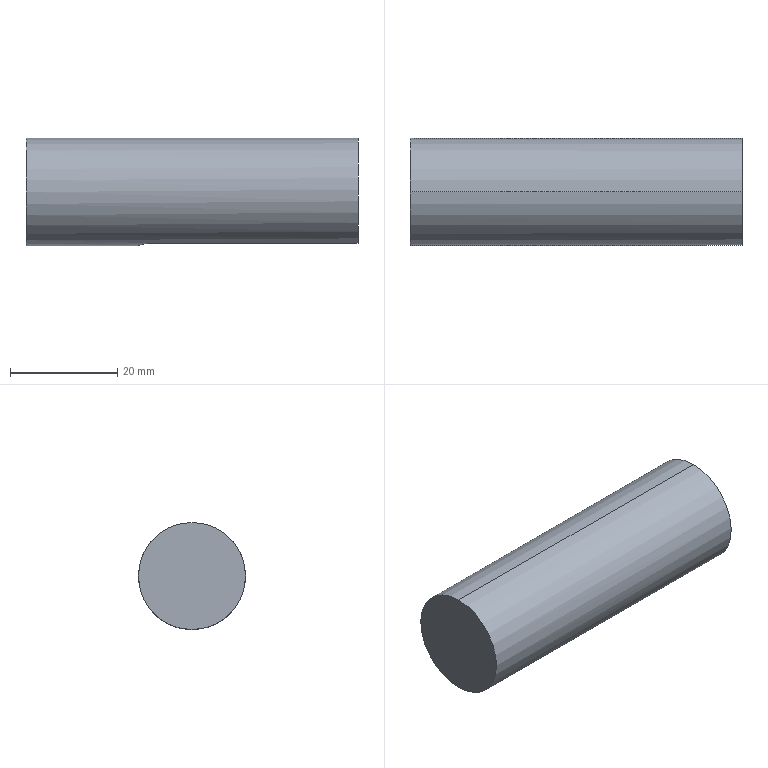Part | STEP file | 0244_Z_102_ARA610LR_2 | 1 solid | 8 faces | box 62 x 20 x 20 mm | volume 18667 mm3 | plane 5 | cylinder 3 | commonest cylinder face diameters 20 x2 6 x1
STEP:
#1=CARTESIAN_POINT('',(0.,0.,0.));
#2=DIRECTION('',(0.,0.,1.));
#3=DIRECTION('',(1.,0.,0.));
#4=AXIS2_PLACEMENT_3D('',#1,#2,#3);
#5=CARTESIAN_POINT('',(24.,3.,-9.539));
#6=VERTEX_POINT('',#5);
#7=CARTESIAN_POINT('',(21.,0.,-10.));
#8=VERTEX_POINT('',#7);
#9=CARTESIAN_POINT('',(24.,3.,-9.539));
#10=CARTESIAN_POINT('',(23.8,3.,-9.539));
#11=CARTESIAN_POINT('',(23.605,2.98,-9.546));
#12=CARTESIAN_POINT('',(23.219,2.903,-9.569));
#13=CARTESIAN_POINT('',(23.028,2.845,-9.587));
#14=CARTESIAN_POINT('',(22.665,2.694,-9.631));
#15=CARTESIAN_POINT('',(22.494,2.602,-9.656));
#16=CARTESIAN_POINT('',(22.168,2.384,-9.712));
#17=CARTESIAN_POINT('',(22.015,2.258,-9.743));
#18=CARTESIAN_POINT('',(21.603,1.845,-9.832));
#19=CARTESIAN_POINT('',(21.38,1.512,-9.892));
#20=CARTESIAN_POINT('',(21.155,0.971,-9.954));
#21=CARTESIAN_POINT('',(21.097,0.7806,-9.971));
#22=CARTESIAN_POINT('',(21.019,0.3926,-9.994));
#23=CARTESIAN_POINT('',(21.,0.197,-10.));
#24=CARTESIAN_POINT('',(21.,0.,-10.));
#25=B_SPLINE_CURVE_WITH_KNOTS('',3,(#9,#10,#11,#12,#13,#14,#15,#16,#17,#18,#19,#20,#21,#22,#23,#24),.UNSPECIFIED.,.F.,.F.,(4,2,2,2,2,2,2,4),(0.,0.0005898,0.00118,0.001769,0.002359,0.003539,0.004128,0.004718),.UNSPECIFIED.);
#26=CARTESIAN_POINT('',(62.,0.,0.));
#27=DIRECTION('',(-1.,0.,0.));
#28=DIRECTION('',(0.,0.,1.));
#29=AXIS2_PLACEMENT_3D('',#26,#27,#28);
#30=CYLINDRICAL_SURFACE('',#29,10.);
#31=CARTESIAN_POINT('',(2.837,38.));
#32=CARTESIAN_POINT('',(2.837,38.036));
#33=CARTESIAN_POINT('',(2.837,38.109));
#34=CARTESIAN_POINT('',(2.838,38.216));
#35=CARTESIAN_POINT('',(2.839,38.323));
#36=CARTESIAN_POINT('',(2.84,38.43));
#37=CARTESIAN_POINT('',(2.842,38.536));
#38=CARTESIAN_POINT('',(2.844,38.641));
#39=CARTESIAN_POINT('',(2.847,38.745));
#40=CARTESIAN_POINT('',(2.85,38.849));
#41=CARTESIAN_POINT('',(2.853,38.952));
#42=CARTESIAN_POINT('',(2.857,39.054));
#43=CARTESIAN_POINT('',(2.861,39.153));
#44=CARTESIAN_POINT('',(2.865,39.251));
#45=CARTESIAN_POINT('',(2.87,39.348));
#46=CARTESIAN_POINT('',(2.875,39.442));
#47=CARTESIAN_POINT('',(2.881,39.534));
#48=CARTESIAN_POINT('',(2.887,39.625));
#49=CARTESIAN_POINT('',(2.893,39.714));
#50=CARTESIAN_POINT('',(2.899,39.8));
#51=CARTESIAN_POINT('',(2.906,39.885));
#52=CARTESIAN_POINT('',(2.913,39.967));
#53=CARTESIAN_POINT('',(2.92,40.046));
#54=CARTESIAN_POINT('',(2.928,40.123));
#55=CARTESIAN_POINT('',(2.936,40.196));
#56=CARTESIAN_POINT('',(2.944,40.267));
#57=CARTESIAN_POINT('',(2.952,40.336));
#58=CARTESIAN_POINT('',(2.961,40.401));
#59=CARTESIAN_POINT('',(2.969,40.464));
#60=CARTESIAN_POINT('',(2.979,40.523));
#61=CARTESIAN_POINT('',(2.988,40.579));
#62=CARTESIAN_POINT('',(2.997,40.632));
#63=CARTESIAN_POINT('',(3.007,40.682));
#64=CARTESIAN_POINT('',(3.016,40.728));
#65=CARTESIAN_POINT('',(3.026,40.771));
#66=CARTESIAN_POINT('',(3.036,40.81));
#67=CARTESIAN_POINT('',(3.046,40.846));
#68=CARTESIAN_POINT('',(3.057,40.878));
#69=CARTESIAN_POINT('',(3.067,40.907));
#70=CARTESIAN_POINT('',(3.078,40.932));
#71=CARTESIAN_POINT('',(3.088,40.953));
#72=CARTESIAN_POINT('',(3.099,40.97));
#73=CARTESIAN_POINT('',(3.109,40.983));
#74=CARTESIAN_POINT('',(3.12,40.993));
#75=CARTESIAN_POINT('',(3.131,40.999));
#76=CARTESIAN_POINT('',(3.138,41.));
#77=CARTESIAN_POINT('',(3.142,41.));
#78=B_SPLINE_CURVE_WITH_KNOTS('',3,(#31,#32,#33,#34,#35,#36,#37,#38,#39,#40,#41,#42,#43,#44,#45,#46,#47,#48,#49,#50,#51,#52,#53,#54,#55,#56,#57,#58,#59,#60,#61,#62,#63,#64,#65,#66,#67,#68,#69,#70,#71,#72,#73,#74,#75,#76,#77),.UNSPECIFIED.,.F.,.F.,(4,1,1,1,1,1,1,1,1,1,1,1,1,1,1,1,1,1,1,1,1,1,1,1,1,1,1,1,1,1,1,1,1,1,1,1,1,1,1,1,1,1,1,1,4),(0.,0.0001072,0.0002145,0.0003217,0.0004289,0.0005362,0.0006434,0.0007506,0.0008579,0.0009651,0.001072,0.00118,0.001287,0.001394,0.001501,0.001608,0.001716,0.001823,0.00193,0.002037,0.002145,0.002252,0.002359,0.002466,0.002574,0.002681,0.002788,0.002895,0.003003,0.00311,0.003217,0.003324,0.003431,0.003539,0.003646,0.003753,0.00386,0.003968,0.004075,0.004182,0.004289,0.004397,0.004504,0.004611,0.004718),.QUASI_UNIFORM_KNOTS.);
#79=(GEOMETRIC_REPRESENTATION_CONTEXT(2)PARAMETRIC_REPRESENTATION_CONTEXT()REPRESENTATION_CONTEXT('',''));
#80=DEFINITIONAL_REPRESENTATION('',(#78),#79);
#81=PCURVE('',#30,#80);
#82=CARTESIAN_POINT('',(24.,0.,-14.5));
#83=DIRECTION('',(0.,0.,1.));
#84=DIRECTION('',(1.,0.,0.));
#85=AXIS2_PLACEMENT_3D('',#82,#83,#84);
#86=CYLINDRICAL_SURFACE('',#85,3.);
#87=CARTESIAN_POINT('',(1.571,4.961));
#88=CARTESIAN_POINT('',(1.583,4.961));
#89=CARTESIAN_POINT('',(1.607,4.96));
#90=CARTESIAN_POINT('',(1.643,4.958));
#91=CARTESIAN_POINT('',(1.679,4.955));
#92=CARTESIAN_POINT('',(1.715,4.951));
#93=CARTESIAN_POINT('',(1.75,4.946));
#94=CARTESIAN_POINT('',(1.786,4.939));
#95=CARTESIAN_POINT('',(1.822,4.932));
#96=CARTESIAN_POINT('',(1.858,4.923));
#97=CARTESIAN_POINT('',(1.894,4.913));
#98=CARTESIAN_POINT('',(1.93,4.903));
#99=CARTESIAN_POINT('',(1.965,4.891));
#100=CARTESIAN_POINT('',(2.001,4.879));
#101=CARTESIAN_POINT('',(2.037,4.866));
#102=CARTESIAN_POINT('',(2.072,4.852));
#103=CARTESIAN_POINT('',(2.107,4.838));
#104=CARTESIAN_POINT('',(2.143,4.823));
#105=CARTESIAN_POINT('',(2.179,4.808));
#106=CARTESIAN_POINT('',(2.214,4.792));
#107=CARTESIAN_POINT('',(2.25,4.776));
#108=CARTESIAN_POINT('',(2.286,4.76));
#109=CARTESIAN_POINT('',(2.321,4.744));
#110=CARTESIAN_POINT('',(2.357,4.727));
#111=CARTESIAN_POINT('',(2.392,4.711));
#112=CARTESIAN_POINT('',(2.427,4.695));
#113=CARTESIAN_POINT('',(2.463,4.679));
#114=CARTESIAN_POINT('',(2.499,4.663));
#115=CARTESIAN_POINT('',(2.534,4.648));
#116=CARTESIAN_POINT('',(2.57,4.633));
#117=CARTESIAN_POINT('',(2.605,4.618));
#118=CARTESIAN_POINT('',(2.641,4.604));
#119=CARTESIAN_POINT('',(2.677,4.591));
#120=CARTESIAN_POINT('',(2.712,4.578));
#121=CARTESIAN_POINT('',(2.748,4.566));
#122=CARTESIAN_POINT('',(2.783,4.555));
#123=CARTESIAN_POINT('',(2.819,4.545));
#124=CARTESIAN_POINT('',(2.855,4.536));
#125=CARTESIAN_POINT('',(2.891,4.528));
#126=CARTESIAN_POINT('',(2.927,4.52));
#127=CARTESIAN_POINT('',(2.963,4.514));
#128=CARTESIAN_POINT('',(2.999,4.509));
#129=CARTESIAN_POINT('',(3.034,4.505));
#130=CARTESIAN_POINT('',(3.07,4.502));
#131=CARTESIAN_POINT('',(3.106,4.5));
#132=CARTESIAN_POINT('',(3.13,4.5));
#133=CARTESIAN_POINT('',(3.142,4.5));
#134=B_SPLINE_CURVE_WITH_KNOTS('',3,(#87,#88,#89,#90,#91,#92,#93,#94,#95,#96,#97,#98,#99,#100,#101,#102,#103,#104,#105,#106,#107,#108,#109,#110,#111,#112,#113,#114,#115,#116,#117,#118,#119,#120,#121,#122,#123,#124,#125,#126,#127,#128,#129,#130,#131,#132,#133),.UNSPECIFIED.,.F.,.F.,(4,1,1,1,1,1,1,1,1,1,1,1,1,1,1,1,1,1,1,1,1,1,1,1,1,1,1,1,1,1,1,1,1,1,1,1,1,1,1,1,1,1,1,1,4),(0.,0.0001072,0.0002145,0.0003217,0.0004289,0.0005362,0.0006434,0.0007506,0.0008579,0.0009651,0.001072,0.00118,0.001287,0.001394,0.001501,0.001608,0.001716,0.001823,0.00193,0.002037,0.002145,0.002252,0.002359,0.002466,0.002574,0.002681,0.002788,0.002895,0.003003,0.00311,0.003217,0.003324,0.003431,0.003539,0.003646,0.003753,0.00386,0.003968,0.004075,0.004182,0.004289,0.004397,0.004504,0.004611,0.004718),.QUASI_UNIFORM_KNOTS.);
#135=(GEOMETRIC_REPRESENTATION_CONTEXT(2)PARAMETRIC_REPRESENTATION_CONTEXT()REPRESENTATION_CONTEXT('',''));
#136=DEFINITIONAL_REPRESENTATION('',(#134),#135);
#137=PCURVE('',#86,#136);
#138=SURFACE_CURVE('',#25,(#81,#137),.PCURVE_S1.);
#139=EDGE_CURVE('',#6,#8,#138,.T.);
#140=ORIENTED_EDGE('',*,*,#139,.T.);
#141=CARTESIAN_POINT('',(0.,0.,-10.));
#142=VERTEX_POINT('',#141);
#143=CARTESIAN_POINT('',(62.,0.,-10.));
#144=DIRECTION('',(-1.,0.,0.));
#145=VECTOR('',#144,1.);
#146=LINE('',#143,#145);
#147=CARTESIAN_POINT('',(3.142,0.));
#148=DIRECTION('',(0.,1.));
#149=VECTOR('',#148,1.);
#150=LINE('',#147,#149);
#151=(GEOMETRIC_REPRESENTATION_CONTEXT(2)PARAMETRIC_REPRESENTATION_CONTEXT()REPRESENTATION_CONTEXT('',''));
#152=DEFINITIONAL_REPRESENTATION('',(#150),#151);
#153=PCURVE('',#30,#152);
#154=CARTESIAN_POINT('',(62.,0.,0.));
#155=DIRECTION('',(-1.,0.,0.));
#156=DIRECTION('',(0.,0.,1.));
#157=AXIS2_PLACEMENT_3D('',#154,#155,#156);
#158=CYLINDRICAL_SURFACE('',#157,10.);
#159=CARTESIAN_POINT('',(3.142,0.));
#160=DIRECTION('',(0.,1.));
#161=VECTOR('',#160,1.);
#162=LINE('',#159,#161);
#163=(GEOMETRIC_REPRESENTATION_CONTEXT(2)PARAMETRIC_REPRESENTATION_CONTEXT()REPRESENTATION_CONTEXT('',''));
#164=DEFINITIONAL_REPRESENTATION('',(#162),#163);
#165=PCURVE('',#158,#164);
#166=SURFACE_CURVE('',#146,(#153,#165),.PCURVE_S1.);
#167=EDGE_CURVE('',#8,#142,#166,.T.);
#168=ORIENTED_EDGE('',*,*,#167,.T.);
#169=CARTESIAN_POINT('',(0.,0.,10.));
#170=VERTEX_POINT('',#169);
#171=CARTESIAN_POINT('',(0.,0.,0.));
#172=DIRECTION('',(-1.,0.,0.));
#173=DIRECTION('',(0.,0.,1.));
#174=AXIS2_PLACEMENT_3D('',#171,#172,#173);
#175=CIRCLE('',#174,10.);
#176=CARTESIAN_POINT('',(0.,62.));
#177=DIRECTION('',(1.,0.));
#178=VECTOR('',#177,1.);
#179=LINE('',#176,#178);
#180=(GEOMETRIC_REPRESENTATION_CONTEXT(2)PARAMETRIC_REPRESENTATION_CONTEXT()REPRESENTATION_CONTEXT('',''));
#181=DEFINITIONAL_REPRESENTATION('',(#179),#180);
#182=PCURVE('',#30,#181);
#183=CARTESIAN_POINT('',(0.,0.,0.));
#184=DIRECTION('',(1.,0.,0.));
#185=DIRECTION('',(0.,0.,-1.));
#186=AXIS2_PLACEMENT_3D('',#183,#184,#185);
#187=PLANE('',#186);
#188=CARTESIAN_POINT('',(-10.,0.));
#189=CARTESIAN_POINT('',(-10.,17.321));
#190=CARTESIAN_POINT('',(5.,8.66));
#191=CARTESIAN_POINT('',(20.,0.));
#192=CARTESIAN_POINT('',(5.,-8.66));
#193=CARTESIAN_POINT('',(-10.,-17.321));
#194=CARTESIAN_POINT('',(-10.,0.));
#195=(BOUNDED_CURVE()B_SPLINE_CURVE(2,(#188,#189,#190,#191,#192,#193,#194),.UNSPECIFIED.,.T.,.F.)B_SPLINE_CURVE_WITH_KNOTS((1,2,2,2,2,1),(-2.094,0.,2.094,4.189,6.283,8.378),.UNSPECIFIED.)CURVE()GEOMETRIC_REPRESENTATION_ITEM()RATIONAL_B_SPLINE_CURVE((1.,0.5,1.,0.5,1.,0.5,1.))REPRESENTATION_ITEM(''));
#196=(GEOMETRIC_REPRESENTATION_CONTEXT(2)PARAMETRIC_REPRESENTATION_CONTEXT()REPRESENTATION_CONTEXT('',''));
#197=DEFINITIONAL_REPRESENTATION('',(#195),#196);
#198=PCURVE('',#187,#197);
#199=SURFACE_CURVE('',#175,(#182,#198),.PCURVE_S1.);
#200=EDGE_CURVE('',#170,#142,#199,.T.);
#201=ORIENTED_EDGE('',*,*,#200,.F.);
#202=CARTESIAN_POINT('',(62.,0.,10.));
#203=VERTEX_POINT('',#202);
#204=CARTESIAN_POINT('',(62.,0.,10.));
#205=DIRECTION('',(-1.,0.,0.));
#206=VECTOR('',#205,1.);
#207=LINE('',#204,#206);
#208=CARTESIAN_POINT('',(0.,0.));
#209=DIRECTION('',(0.,1.));
#210=VECTOR('',#209,1.);
#211=LINE('',#208,#210);
#212=(GEOMETRIC_REPRESENTATION_CONTEXT(2)PARAMETRIC_REPRESENTATION_CONTEXT()REPRESENTATION_CONTEXT('',''));
#213=DEFINITIONAL_REPRESENTATION('',(#211),#212);
#214=PCURVE('',#30,#213);
#215=CARTESIAN_POINT('',(6.283,0.));
#216=DIRECTION('',(0.,1.));
#217=VECTOR('',#216,1.);
#218=LINE('',#215,#217);
#219=(GEOMETRIC_REPRESENTATION_CONTEXT(2)PARAMETRIC_REPRESENTATION_CONTEXT()REPRESENTATION_CONTEXT('',''));
#220=DEFINITIONAL_REPRESENTATION('',(#218),#219);
#221=PCURVE('',#158,#220);
#222=SURFACE_CURVE('',#207,(#214,#221),.PCURVE_S1.);
#223=EDGE_CURVE('',#203,#170,#222,.T.);
#224=ORIENTED_EDGE('',*,*,#223,.F.);
#225=CARTESIAN_POINT('',(62.,3.,-9.539));
#226=VERTEX_POINT('',#225);
#227=CARTESIAN_POINT('',(62.,0.,0.));
#228=DIRECTION('',(-1.,0.,0.));
#229=DIRECTION('',(0.,0.,1.));
#230=AXIS2_PLACEMENT_3D('',#227,#228,#229);
#231=CIRCLE('',#230,10.);
#232=CARTESIAN_POINT('',(0.,0.));
#233=DIRECTION('',(1.,0.));
#234=VECTOR('',#233,1.);
#235=LINE('',#232,#234);
#236=(GEOMETRIC_REPRESENTATION_CONTEXT(2)PARAMETRIC_REPRESENTATION_CONTEXT()REPRESENTATION_CONTEXT('',''));
#237=DEFINITIONAL_REPRESENTATION('',(#235),#236);
#238=PCURVE('',#30,#237);
#239=CARTESIAN_POINT('',(62.,10.,0.));
#240=DIRECTION('',(-1.,0.,0.));
#241=DIRECTION('',(0.,0.,1.));
#242=AXIS2_PLACEMENT_3D('',#239,#240,#241);
#243=PLANE('',#242);
#244=CARTESIAN_POINT('',(0.,-10.));
#245=DIRECTION('',(1.,0.));
#246=AXIS2_PLACEMENT_2D('',#244,#245);
#247=CIRCLE('',#246,10.);
#248=(GEOMETRIC_REPRESENTATION_CONTEXT(2)PARAMETRIC_REPRESENTATION_CONTEXT()REPRESENTATION_CONTEXT('',''));
#249=DEFINITIONAL_REPRESENTATION('',(#247),#248);
#250=PCURVE('',#243,#249);
#251=SURFACE_CURVE('',#231,(#238,#250),.PCURVE_S1.);
#252=EDGE_CURVE('',#203,#226,#251,.T.);
#253=ORIENTED_EDGE('',*,*,#252,.T.);
#254=CARTESIAN_POINT('',(62.,3.,-9.539));
#255=DIRECTION('',(-1.,0.,0.));
#256=VECTOR('',#255,1.);
#257=LINE('',#254,#256);
#258=CARTESIAN_POINT('',(2.837,0.));
#259=DIRECTION('',(0.,1.));
#260=VECTOR('',#259,1.);
#261=LINE('',#258,#260);
#262=(GEOMETRIC_REPRESENTATION_CONTEXT(2)PARAMETRIC_REPRESENTATION_CONTEXT()REPRESENTATION_CONTEXT('',''));
#263=DEFINITIONAL_REPRESENTATION('',(#261),#262);
#264=PCURVE('',#30,#263);
#265=CARTESIAN_POINT('',(62.,3.,-14.5));
#266=DIRECTION('',(0.,1.,0.));
#267=DIRECTION('',(-1.,0.,0.));
#268=AXIS2_PLACEMENT_3D('',#265,#266,#267);
#269=PLANE('',#268);
#270=CARTESIAN_POINT('',(0.,4.961));
#271=DIRECTION('',(1.,0.));
#272=VECTOR('',#271,1.);
#273=LINE('',#270,#272);
#274=(GEOMETRIC_REPRESENTATION_CONTEXT(2)PARAMETRIC_REPRESENTATION_CONTEXT()REPRESENTATION_CONTEXT('',''));
#275=DEFINITIONAL_REPRESENTATION('',(#273),#274);
#276=PCURVE('',#269,#275);
#277=SURFACE_CURVE('',#257,(#264,#276),.PCURVE_S1.);
#278=EDGE_CURVE('',#226,#6,#277,.T.);
#279=ORIENTED_EDGE('',*,*,#278,.T.);
#280=EDGE_LOOP('',(#140,#168,#201,#224,#253,#279));
#281=FACE_BOUND('',#280,.T.);
#282=ADVANCED_FACE('',(#281),#30,.T.);
#283=ORIENTED_EDGE('',*,*,#200,.T.);
#284=CARTESIAN_POINT('',(0.,0.,0.));
#285=DIRECTION('',(-1.,0.,0.));
#286=DIRECTION('',(0.,0.,1.));
#287=AXIS2_PLACEMENT_3D('',#284,#285,#286);
#288=CIRCLE('',#287,10.);
#289=CARTESIAN_POINT('',(-10.,0.));
#290=CARTESIAN_POINT('',(-10.,17.321));
#291=CARTESIAN_POINT('',(5.,8.66));
#292=CARTESIAN_POINT('',(20.,0.));
#293=CARTESIAN_POINT('',(5.,-8.66));
#294=CARTESIAN_POINT('',(-10.,-17.321));
#295=CARTESIAN_POINT('',(-10.,0.));
#296=(BOUNDED_CURVE()B_SPLINE_CURVE(2,(#289,#290,#291,#292,#293,#294,#295),.UNSPECIFIED.,.T.,.F.)B_SPLINE_CURVE_WITH_KNOTS((1,2,2,2,2,1),(-2.094,0.,2.094,4.189,6.283,8.378),.UNSPECIFIED.)CURVE()GEOMETRIC_REPRESENTATION_ITEM()RATIONAL_B_SPLINE_CURVE((1.,0.5,1.,0.5,1.,0.5,1.))REPRESENTATION_ITEM(''));
#297=(GEOMETRIC_REPRESENTATION_CONTEXT(2)PARAMETRIC_REPRESENTATION_CONTEXT()REPRESENTATION_CONTEXT('',''));
#298=DEFINITIONAL_REPRESENTATION('',(#296),#297);
#299=PCURVE('',#187,#298);
#300=CARTESIAN_POINT('',(0.,62.));
#301=DIRECTION('',(1.,0.));
#302=VECTOR('',#301,1.);
#303=LINE('',#300,#302);
#304=(GEOMETRIC_REPRESENTATION_CONTEXT(2)PARAMETRIC_REPRESENTATION_CONTEXT()REPRESENTATION_CONTEXT('',''));
#305=DEFINITIONAL_REPRESENTATION('',(#303),#304);
#306=PCURVE('',#158,#305);
#307=SURFACE_CURVE('',#288,(#299,#306),.PCURVE_S1.);
#308=EDGE_CURVE('',#142,#170,#307,.T.);
#309=ORIENTED_EDGE('',*,*,#308,.T.);
#310=EDGE_LOOP('',(#283,#309));
#311=FACE_BOUND('',#310,.T.);
#312=ADVANCED_FACE('',(#311),#187,.F.);
#313=ORIENTED_EDGE('',*,*,#167,.F.);
#314=CARTESIAN_POINT('',(24.,-3.,-9.539));
#315=VERTEX_POINT('',#314);
#316=CARTESIAN_POINT('',(21.,0.,-10.));
#317=CARTESIAN_POINT('',(21.,-0.1968,-10.));
#318=CARTESIAN_POINT('',(21.02,-0.3967,-9.994));
#319=CARTESIAN_POINT('',(21.097,-0.7821,-9.971));
#320=CARTESIAN_POINT('',(21.154,-0.9695,-9.955));
#321=CARTESIAN_POINT('',(21.306,-1.334,-9.912));
#322=CARTESIAN_POINT('',(21.399,-1.507,-9.887));
#323=CARTESIAN_POINT('',(21.616,-1.831,-9.832));
#324=CARTESIAN_POINT('',(21.741,-1.983,-9.802));
#325=CARTESIAN_POINT('',(22.017,-2.26,-9.742));
#326=CARTESIAN_POINT('',(22.167,-2.383,-9.713));
#327=CARTESIAN_POINT('',(22.491,-2.6,-9.657));
#328=CARTESIAN_POINT('',(22.667,-2.694,-9.63));
#329=CARTESIAN_POINT('',(23.028,-2.845,-9.587));
#330=CARTESIAN_POINT('',(23.215,-2.902,-9.57));
#331=CARTESIAN_POINT('',(23.601,-2.98,-9.546));
#332=CARTESIAN_POINT('',(23.801,-3.,-9.539));
#333=CARTESIAN_POINT('',(24.,-3.,-9.539));
#334=B_SPLINE_CURVE_WITH_KNOTS('',3,(#316,#317,#318,#319,#320,#321,#322,#323,#324,#325,#326,#327,#328,#329,#330,#331,#332,#333),.UNSPECIFIED.,.F.,.F.,(4,2,2,2,2,2,2,2,4),(0.004718,0.005307,0.005896,0.006485,0.007074,0.007663,0.008252,0.008842,0.009431),.UNSPECIFIED.);
#335=CARTESIAN_POINT('',(3.142,41.));
#336=CARTESIAN_POINT('',(3.145,41.));
#337=CARTESIAN_POINT('',(3.152,40.999));
#338=CARTESIAN_POINT('',(3.163,40.993));
#339=CARTESIAN_POINT('',(3.174,40.983));
#340=CARTESIAN_POINT('',(3.185,40.97));
#341=CARTESIAN_POINT('',(3.195,40.952));
#342=CARTESIAN_POINT('',(3.206,40.931));
#343=CARTESIAN_POINT('',(3.216,40.906));
#344=CARTESIAN_POINT('',(3.227,40.878));
#345=CARTESIAN_POINT('',(3.237,40.846));
#346=CARTESIAN_POINT('',(3.247,40.81));
#347=CARTESIAN_POINT('',(3.257,40.771));
#348=CARTESIAN_POINT('',(3.267,40.728));
#349=CARTESIAN_POINT('',(3.277,40.681));
#350=CARTESIAN_POINT('',(3.286,40.631));
#351=CARTESIAN_POINT('',(3.296,40.578));
#352=CARTESIAN_POINT('',(3.305,40.522));
#353=CARTESIAN_POINT('',(3.314,40.463));
#354=CARTESIAN_POINT('',(3.323,40.401));
#355=CARTESIAN_POINT('',(3.331,40.335));
#356=CARTESIAN_POINT('',(3.339,40.267));
#357=CARTESIAN_POINT('',(3.348,40.196));
#358=CARTESIAN_POINT('',(3.355,40.121));
#359=CARTESIAN_POINT('',(3.363,40.045));
#360=CARTESIAN_POINT('',(3.37,39.966));
#361=CARTESIAN_POINT('',(3.377,39.884));
#362=CARTESIAN_POINT('',(3.384,39.801));
#363=CARTESIAN_POINT('',(3.39,39.715));
#364=CARTESIAN_POINT('',(3.396,39.627));
#365=CARTESIAN_POINT('',(3.402,39.536));
#366=CARTESIAN_POINT('',(3.408,39.443));
#367=CARTESIAN_POINT('',(3.413,39.348));
#368=CARTESIAN_POINT('',(3.418,39.251));
#369=CARTESIAN_POINT('',(3.422,39.153));
#370=CARTESIAN_POINT('',(3.426,39.054));
#371=CARTESIAN_POINT('',(3.43,38.954));
#372=CARTESIAN_POINT('',(3.433,38.852));
#373=CARTESIAN_POINT('',(3.436,38.749));
#374=CARTESIAN_POINT('',(3.439,38.645));
#375=CARTESIAN_POINT('',(3.441,38.539));
#376=CARTESIAN_POINT('',(3.443,38.433));
#377=CARTESIAN_POINT('',(3.444,38.325));
#378=CARTESIAN_POINT('',(3.446,38.217));
#379=CARTESIAN_POINT('',(3.446,38.109));
#380=CARTESIAN_POINT('',(3.446,38.036));
#381=CARTESIAN_POINT('',(3.446,38.));
#382=B_SPLINE_CURVE_WITH_KNOTS('',3,(#335,#336,#337,#338,#339,#340,#341,#342,#343,#344,#345,#346,#347,#348,#349,#350,#351,#352,#353,#354,#355,#356,#357,#358,#359,#360,#361,#362,#363,#364,#365,#366,#367,#368,#369,#370,#371,#372,#373,#374,#375,#376,#377,#378,#379,#380,#381),.UNSPECIFIED.,.F.,.F.,(4,1,1,1,1,1,1,1,1,1,1,1,1,1,1,1,1,1,1,1,1,1,1,1,1,1,1,1,1,1,1,1,1,1,1,1,1,1,1,1,1,1,1,1,4),(0.004718,0.004825,0.004932,0.00504,0.005147,0.005254,0.005361,0.005468,0.005575,0.005682,0.005789,0.005896,0.006003,0.006111,0.006218,0.006325,0.006432,0.006539,0.006646,0.006753,0.00686,0.006967,0.007074,0.007181,0.007289,0.007396,0.007503,0.00761,0.007717,0.007824,0.007931,0.008038,0.008145,0.008252,0.00836,0.008467,0.008574,0.008681,0.008788,0.008895,0.009002,0.009109,0.009216,0.009323,0.009431),.QUASI_UNIFORM_KNOTS.);
#383=(GEOMETRIC_REPRESENTATION_CONTEXT(2)PARAMETRIC_REPRESENTATION_CONTEXT()REPRESENTATION_CONTEXT('',''));
#384=DEFINITIONAL_REPRESENTATION('',(#382),#383);
#385=PCURVE('',#158,#384);
#386=CARTESIAN_POINT('',(3.142,4.5));
#387=CARTESIAN_POINT('',(3.154,4.5));
#388=CARTESIAN_POINT('',(3.177,4.5));
#389=CARTESIAN_POINT('',(3.213,4.502));
#390=CARTESIAN_POINT('',(3.25,4.505));
#391=CARTESIAN_POINT('',(3.286,4.509));
#392=CARTESIAN_POINT('',(3.321,4.514));
#393=CARTESIAN_POINT('',(3.357,4.52));
#394=CARTESIAN_POINT('',(3.393,4.528));
#395=CARTESIAN_POINT('',(3.428,4.536));
#396=CARTESIAN_POINT('',(3.464,4.545));
#397=CARTESIAN_POINT('',(3.5,4.555));
#398=CARTESIAN_POINT('',(3.536,4.566));
#399=CARTESIAN_POINT('',(3.571,4.578));
#400=CARTESIAN_POINT('',(3.607,4.591));
#401=CARTESIAN_POINT('',(3.643,4.604));
#402=CARTESIAN_POINT('',(3.678,4.618));
#403=CARTESIAN_POINT('',(3.714,4.633));
#404=CARTESIAN_POINT('',(3.749,4.648));
#405=CARTESIAN_POINT('',(3.785,4.663));
#406=CARTESIAN_POINT('',(3.82,4.679));
#407=CARTESIAN_POINT('',(3.856,4.695));
#408=CARTESIAN_POINT('',(3.892,4.711));
#409=CARTESIAN_POINT('',(3.927,4.728));
#410=CARTESIAN_POINT('',(3.963,4.744));
#411=CARTESIAN_POINT('',(3.998,4.76));
#412=CARTESIAN_POINT('',(4.033,4.776));
#413=CARTESIAN_POINT('',(4.069,4.792));
#414=CARTESIAN_POINT('',(4.104,4.808));
#415=CARTESIAN_POINT('',(4.139,4.823));
#416=CARTESIAN_POINT('',(4.175,4.838));
#417=CARTESIAN_POINT('',(4.211,4.852));
#418=CARTESIAN_POINT('',(4.247,4.866));
#419=CARTESIAN_POINT('',(4.282,4.879));
#420=CARTESIAN_POINT('',(4.318,4.891));
#421=CARTESIAN_POINT('',(4.353,4.903));
#422=CARTESIAN_POINT('',(4.389,4.913));
#423=CARTESIAN_POINT('',(4.424,4.923));
#424=CARTESIAN_POINT('',(4.46,4.931));
#425=CARTESIAN_POINT('',(4.496,4.939));
#426=CARTESIAN_POINT('',(4.532,4.946));
#427=CARTESIAN_POINT('',(4.568,4.951));
#428=CARTESIAN_POINT('',(4.604,4.955));
#429=CARTESIAN_POINT('',(4.64,4.958));
#430=CARTESIAN_POINT('',(4.676,4.96));
#431=CARTESIAN_POINT('',(4.7,4.961));
#432=CARTESIAN_POINT('',(4.712,4.961));
#433=B_SPLINE_CURVE_WITH_KNOTS('',3,(#386,#387,#388,#389,#390,#391,#392,#393,#394,#395,#396,#397,#398,#399,#400,#401,#402,#403,#404,#405,#406,#407,#408,#409,#410,#411,#412,#413,#414,#415,#416,#417,#418,#419,#420,#421,#422,#423,#424,#425,#426,#427,#428,#429,#430,#431,#432),.UNSPECIFIED.,.F.,.F.,(4,1,1,1,1,1,1,1,1,1,1,1,1,1,1,1,1,1,1,1,1,1,1,1,1,1,1,1,1,1,1,1,1,1,1,1,1,1,1,1,1,1,1,1,4),(0.004718,0.004825,0.004932,0.00504,0.005147,0.005254,0.005361,0.005468,0.005575,0.005682,0.005789,0.005896,0.006003,0.006111,0.006218,0.006325,0.006432,0.006539,0.006646,0.006753,0.00686,0.006967,0.007074,0.007181,0.007289,0.007396,0.007503,0.00761,0.007717,0.007824,0.007931,0.008038,0.008145,0.008252,0.00836,0.008467,0.008574,0.008681,0.008788,0.008895,0.009002,0.009109,0.009216,0.009323,0.009431),.QUASI_UNIFORM_KNOTS.);
#434=(GEOMETRIC_REPRESENTATION_CONTEXT(2)PARAMETRIC_REPRESENTATION_CONTEXT()REPRESENTATION_CONTEXT('',''));
#435=DEFINITIONAL_REPRESENTATION('',(#433),#434);
#436=PCURVE('',#86,#435);
#437=SURFACE_CURVE('',#334,(#385,#436),.PCURVE_S1.);
#438=EDGE_CURVE('',#8,#315,#437,.T.);
#439=ORIENTED_EDGE('',*,*,#438,.T.);
#440=CARTESIAN_POINT('',(62.,-3.,-9.539));
#441=VERTEX_POINT('',#440);
#442=CARTESIAN_POINT('',(62.,-3.,-9.539));
#443=DIRECTION('',(1.,0.,0.));
#444=VECTOR('',#443,1.);
#445=LINE('',#442,#444);
#446=CARTESIAN_POINT('',(3.446,0.));
#447=DIRECTION('',(0.,-1.));
#448=VECTOR('',#447,1.);
#449=LINE('',#446,#448);
#450=(GEOMETRIC_REPRESENTATION_CONTEXT(2)PARAMETRIC_REPRESENTATION_CONTEXT()REPRESENTATION_CONTEXT('',''));
#451=DEFINITIONAL_REPRESENTATION('',(#449),#450);
#452=PCURVE('',#158,#451);
#453=CARTESIAN_POINT('',(24.,-3.,-14.5));
#454=DIRECTION('',(0.,-1.,0.));
#455=DIRECTION('',(0.,0.,-1.));
#456=AXIS2_PLACEMENT_3D('',#453,#454,#455);
#457=PLANE('',#456);
#458=CARTESIAN_POINT('',(-4.961,38.));
#459=DIRECTION('',(0.,1.));
#460=VECTOR('',#459,1.);
#461=LINE('',#458,#460);
#462=(GEOMETRIC_REPRESENTATION_CONTEXT(2)PARAMETRIC_REPRESENTATION_CONTEXT()REPRESENTATION_CONTEXT('',''));
#463=DEFINITIONAL_REPRESENTATION('',(#461),#462);
#464=PCURVE('',#457,#463);
#465=SURFACE_CURVE('',#445,(#452,#464),.PCURVE_S1.);
#466=EDGE_CURVE('',#315,#441,#465,.T.);
#467=ORIENTED_EDGE('',*,*,#466,.T.);
#468=CARTESIAN_POINT('',(62.,0.,0.));
#469=DIRECTION('',(-1.,0.,0.));
#470=DIRECTION('',(0.,0.,1.));
#471=AXIS2_PLACEMENT_3D('',#468,#469,#470);
#472=CIRCLE('',#471,10.);
#473=CARTESIAN_POINT('',(0.,0.));
#474=DIRECTION('',(1.,0.));
#475=VECTOR('',#474,1.);
#476=LINE('',#473,#475);
#477=(GEOMETRIC_REPRESENTATION_CONTEXT(2)PARAMETRIC_REPRESENTATION_CONTEXT()REPRESENTATION_CONTEXT('',''));
#478=DEFINITIONAL_REPRESENTATION('',(#476),#477);
#479=PCURVE('',#158,#478);
#480=CARTESIAN_POINT('',(0.,-10.));
#481=DIRECTION('',(1.,0.));
#482=AXIS2_PLACEMENT_2D('',#480,#481);
#483=CIRCLE('',#482,10.);
#484=(GEOMETRIC_REPRESENTATION_CONTEXT(2)PARAMETRIC_REPRESENTATION_CONTEXT()REPRESENTATION_CONTEXT('',''));
#485=DEFINITIONAL_REPRESENTATION('',(#483),#484);
#486=PCURVE('',#243,#485);
#487=SURFACE_CURVE('',#472,(#479,#486),.PCURVE_S1.);
#488=EDGE_CURVE('',#441,#203,#487,.T.);
#489=ORIENTED_EDGE('',*,*,#488,.T.);
#490=ORIENTED_EDGE('',*,*,#223,.T.);
#491=ORIENTED_EDGE('',*,*,#308,.F.);
#492=EDGE_LOOP('',(#313,#439,#467,#489,#490,#491));
#493=FACE_BOUND('',#492,.T.);
#494=ADVANCED_FACE('',(#493),#158,.T.);
#495=CARTESIAN_POINT('',(62.,-3.,-6.5));
#496=VERTEX_POINT('',#495);
#497=CARTESIAN_POINT('',(62.,3.,-6.5));
#498=VERTEX_POINT('',#497);
#499=CARTESIAN_POINT('',(62.,-3.,-6.5));
#500=DIRECTION('',(0.,1.,0.));
#501=VECTOR('',#500,1.);
#502=LINE('',#499,#501);
#503=CARTESIAN_POINT('',(-6.5,-13.));
#504=DIRECTION('',(0.,1.));
#505=VECTOR('',#504,1.);
#506=LINE('',#503,#505);
#507=(GEOMETRIC_REPRESENTATION_CONTEXT(2)PARAMETRIC_REPRESENTATION_CONTEXT()REPRESENTATION_CONTEXT('',''));
#508=DEFINITIONAL_REPRESENTATION('',(#506),#507);
#509=PCURVE('',#243,#508);
#510=CARTESIAN_POINT('',(24.,0.,-6.5));
#511=DIRECTION('',(0.,0.,1.));
#512=DIRECTION('',(1.,0.,0.));
#513=AXIS2_PLACEMENT_3D('',#510,#511,#512);
#514=PLANE('',#513);
#515=CARTESIAN_POINT('',(38.,-3.));
#516=DIRECTION('',(0.,1.));
#517=VECTOR('',#516,1.);
#518=LINE('',#515,#517);
#519=(GEOMETRIC_REPRESENTATION_CONTEXT(2)PARAMETRIC_REPRESENTATION_CONTEXT()REPRESENTATION_CONTEXT('',''));
#520=DEFINITIONAL_REPRESENTATION('',(#518),#519);
#521=PCURVE('',#514,#520);
#522=SURFACE_CURVE('',#502,(#509,#521),.PCURVE_S1.);
#523=EDGE_CURVE('',#496,#498,#522,.T.);
#524=ORIENTED_EDGE('',*,*,#523,.T.);
#525=CARTESIAN_POINT('',(62.,3.,0.));
#526=DIRECTION('',(0.,0.,-1.));
#527=VECTOR('',#526,1.);
#528=LINE('',#525,#527);
#529=CARTESIAN_POINT('',(0.,-7.));
#530=DIRECTION('',(-1.,0.));
#531=VECTOR('',#530,1.);
#532=LINE('',#529,#531);
#533=(GEOMETRIC_REPRESENTATION_CONTEXT(2)PARAMETRIC_REPRESENTATION_CONTEXT()REPRESENTATION_CONTEXT('',''));
#534=DEFINITIONAL_REPRESENTATION('',(#532),#533);
#535=PCURVE('',#243,#534);
#536=CARTESIAN_POINT('',(0.,14.5));
#537=DIRECTION('',(0.,-1.));
#538=VECTOR('',#537,1.);
#539=LINE('',#536,#538);
#540=(GEOMETRIC_REPRESENTATION_CONTEXT(2)PARAMETRIC_REPRESENTATION_CONTEXT()REPRESENTATION_CONTEXT('',''));
#541=DEFINITIONAL_REPRESENTATION('',(#539),#540);
#542=PCURVE('',#269,#541);
#543=SURFACE_CURVE('',#528,(#535,#542),.PCURVE_S1.);
#544=EDGE_CURVE('',#498,#226,#543,.T.);
#545=ORIENTED_EDGE('',*,*,#544,.T.);
#546=ORIENTED_EDGE('',*,*,#252,.F.);
#547=ORIENTED_EDGE('',*,*,#488,.F.);
#548=CARTESIAN_POINT('',(62.,-3.,0.));
#549=DIRECTION('',(0.,0.,1.));
#550=VECTOR('',#549,1.);
#551=LINE('',#548,#550);
#552=CARTESIAN_POINT('',(0.,-13.));
#553=DIRECTION('',(1.,0.));
#554=VECTOR('',#553,1.);
#555=LINE('',#552,#554);
#556=(GEOMETRIC_REPRESENTATION_CONTEXT(2)PARAMETRIC_REPRESENTATION_CONTEXT()REPRESENTATION_CONTEXT('',''));
#557=DEFINITIONAL_REPRESENTATION('',(#555),#556);
#558=PCURVE('',#243,#557);
#559=CARTESIAN_POINT('',(-14.5,38.));
#560=DIRECTION('',(-1.,0.));
#561=VECTOR('',#560,1.);
#562=LINE('',#559,#561);
#563=(GEOMETRIC_REPRESENTATION_CONTEXT(2)PARAMETRIC_REPRESENTATION_CONTEXT()REPRESENTATION_CONTEXT('',''));
#564=DEFINITIONAL_REPRESENTATION('',(#562),#563);
#565=PCURVE('',#457,#564);
#566=SURFACE_CURVE('',#551,(#558,#565),.PCURVE_S1.);
#567=EDGE_CURVE('',#441,#496,#566,.T.);
#568=ORIENTED_EDGE('',*,*,#567,.T.);
#569=EDGE_LOOP('',(#524,#545,#546,#547,#568));
#570=FACE_BOUND('',#569,.T.);
#571=ADVANCED_FACE('',(#570),#243,.F.);
#572=ORIENTED_EDGE('',*,*,#139,.T.);
#573=ORIENTED_EDGE('',*,*,#438,.T.);
#574=CARTESIAN_POINT('',(24.,-3.,-6.5));
#575=VERTEX_POINT('',#574);
#576=CARTESIAN_POINT('',(24.,-3.,-14.5));
#577=DIRECTION('',(0.,0.,1.));
#578=VECTOR('',#577,1.);
#579=LINE('',#576,#578);
#580=CARTESIAN_POINT('',(4.712,0.));
#581=DIRECTION('',(0.,1.));
#582=VECTOR('',#581,1.);
#583=LINE('',#580,#582);
#584=(GEOMETRIC_REPRESENTATION_CONTEXT(2)PARAMETRIC_REPRESENTATION_CONTEXT()REPRESENTATION_CONTEXT('',''));
#585=DEFINITIONAL_REPRESENTATION('',(#583),#584);
#586=PCURVE('',#86,#585);
#587=CARTESIAN_POINT('',(0.,0.));
#588=DIRECTION('',(-1.,0.));
#589=VECTOR('',#588,1.);
#590=LINE('',#587,#589);
#591=(GEOMETRIC_REPRESENTATION_CONTEXT(2)PARAMETRIC_REPRESENTATION_CONTEXT()REPRESENTATION_CONTEXT('',''));
#592=DEFINITIONAL_REPRESENTATION('',(#590),#591);
#593=PCURVE('',#457,#592);
#594=SURFACE_CURVE('',#579,(#586,#593),.PCURVE_S1.);
#595=EDGE_CURVE('',#315,#575,#594,.T.);
#596=ORIENTED_EDGE('',*,*,#595,.T.);
#597=CARTESIAN_POINT('',(24.,3.,-6.5));
#598=VERTEX_POINT('',#597);
#599=CARTESIAN_POINT('',(24.,0.,-6.5));
#600=DIRECTION('',(0.,0.,1.));
#601=DIRECTION('',(1.,0.,0.));
#602=AXIS2_PLACEMENT_3D('',#599,#600,#601);
#603=CIRCLE('',#602,3.);
#604=CARTESIAN_POINT('',(0.,8.));
#605=DIRECTION('',(1.,0.));
#606=VECTOR('',#605,1.);
#607=LINE('',#604,#606);
#608=(GEOMETRIC_REPRESENTATION_CONTEXT(2)PARAMETRIC_REPRESENTATION_CONTEXT()REPRESENTATION_CONTEXT('',''));
#609=DEFINITIONAL_REPRESENTATION('',(#607),#608);
#610=PCURVE('',#86,#609);
#611=CARTESIAN_POINT('',(0.,0.));
#612=DIRECTION('',(1.,0.));
#613=AXIS2_PLACEMENT_2D('',#611,#612);
#614=CIRCLE('',#613,3.);
#615=(GEOMETRIC_REPRESENTATION_CONTEXT(2)PARAMETRIC_REPRESENTATION_CONTEXT()REPRESENTATION_CONTEXT('',''));
#616=DEFINITIONAL_REPRESENTATION('',(#614),#615);
#617=PCURVE('',#514,#616);
#618=SURFACE_CURVE('',#603,(#610,#617),.PCURVE_S1.);
#619=EDGE_CURVE('',#598,#575,#618,.T.);
#620=ORIENTED_EDGE('',*,*,#619,.F.);
#621=CARTESIAN_POINT('',(24.,3.,-14.5));
#622=DIRECTION('',(0.,0.,1.));
#623=VECTOR('',#622,1.);
#624=LINE('',#621,#623);
#625=CARTESIAN_POINT('',(1.571,0.));
#626=DIRECTION('',(0.,1.));
#627=VECTOR('',#626,1.);
#628=LINE('',#625,#627);
#629=(GEOMETRIC_REPRESENTATION_CONTEXT(2)PARAMETRIC_REPRESENTATION_CONTEXT()REPRESENTATION_CONTEXT('',''));
#630=DEFINITIONAL_REPRESENTATION('',(#628),#629);
#631=PCURVE('',#86,#630);
#632=CARTESIAN_POINT('',(38.,0.));
#633=DIRECTION('',(0.,1.));
#634=VECTOR('',#633,1.);
#635=LINE('',#632,#634);
#636=(GEOMETRIC_REPRESENTATION_CONTEXT(2)PARAMETRIC_REPRESENTATION_CONTEXT()REPRESENTATION_CONTEXT('',''));
#637=DEFINITIONAL_REPRESENTATION('',(#635),#636);
#638=PCURVE('',#269,#637);
#639=SURFACE_CURVE('',#624,(#631,#638),.PCURVE_S1.);
#640=EDGE_CURVE('',#6,#598,#639,.T.);
#641=ORIENTED_EDGE('',*,*,#640,.F.);
#642=EDGE_LOOP('',(#572,#573,#596,#620,#641));
#643=FACE_BOUND('',#642,.F.);
#644=ADVANCED_FACE('',(#643),#86,.F.);
#645=ORIENTED_EDGE('',*,*,#544,.F.);
#646=CARTESIAN_POINT('',(62.,3.,-6.5));
#647=DIRECTION('',(-1.,0.,0.));
#648=VECTOR('',#647,1.);
#649=LINE('',#646,#648);
#650=CARTESIAN_POINT('',(0.,8.));
#651=DIRECTION('',(1.,0.));
#652=VECTOR('',#651,1.);
#653=LINE('',#650,#652);
#654=(GEOMETRIC_REPRESENTATION_CONTEXT(2)PARAMETRIC_REPRESENTATION_CONTEXT()REPRESENTATION_CONTEXT('',''));
#655=DEFINITIONAL_REPRESENTATION('',(#653),#654);
#656=PCURVE('',#269,#655);
#657=CARTESIAN_POINT('',(38.,3.));
#658=DIRECTION('',(-1.,0.));
#659=VECTOR('',#658,1.);
#660=LINE('',#657,#659);
#661=(GEOMETRIC_REPRESENTATION_CONTEXT(2)PARAMETRIC_REPRESENTATION_CONTEXT()REPRESENTATION_CONTEXT('',''));
#662=DEFINITIONAL_REPRESENTATION('',(#660),#661);
#663=PCURVE('',#514,#662);
#664=SURFACE_CURVE('',#649,(#656,#663),.PCURVE_S1.);
#665=EDGE_CURVE('',#498,#598,#664,.T.);
#666=ORIENTED_EDGE('',*,*,#665,.T.);
#667=ORIENTED_EDGE('',*,*,#640,.F.);
#668=ORIENTED_EDGE('',*,*,#278,.F.);
#669=EDGE_LOOP('',(#645,#666,#667,#668));
#670=FACE_BOUND('',#669,.T.);
#671=ADVANCED_FACE('',(#670),#269,.F.);
#672=ORIENTED_EDGE('',*,*,#595,.T.);
#673=CARTESIAN_POINT('',(24.,-3.,-6.5));
#674=DIRECTION('',(1.,0.,0.));
#675=VECTOR('',#674,1.);
#676=LINE('',#673,#675);
#677=CARTESIAN_POINT('',(-8.,0.));
#678=DIRECTION('',(0.,1.));
#679=VECTOR('',#678,1.);
#680=LINE('',#677,#679);
#681=(GEOMETRIC_REPRESENTATION_CONTEXT(2)PARAMETRIC_REPRESENTATION_CONTEXT()REPRESENTATION_CONTEXT('',''));
#682=DEFINITIONAL_REPRESENTATION('',(#680),#681);
#683=PCURVE('',#457,#682);
#684=CARTESIAN_POINT('',(0.,-3.));
#685=DIRECTION('',(1.,0.));
#686=VECTOR('',#685,1.);
#687=LINE('',#684,#686);
#688=(GEOMETRIC_REPRESENTATION_CONTEXT(2)PARAMETRIC_REPRESENTATION_CONTEXT()REPRESENTATION_CONTEXT('',''));
#689=DEFINITIONAL_REPRESENTATION('',(#687),#688);
#690=PCURVE('',#514,#689);
#691=SURFACE_CURVE('',#676,(#683,#690),.PCURVE_S1.);
#692=EDGE_CURVE('',#575,#496,#691,.T.);
#693=ORIENTED_EDGE('',*,*,#692,.T.);
#694=ORIENTED_EDGE('',*,*,#567,.F.);
#695=ORIENTED_EDGE('',*,*,#466,.F.);
#696=EDGE_LOOP('',(#672,#693,#694,#695));
#697=FACE_BOUND('',#696,.T.);
#698=ADVANCED_FACE('',(#697),#457,.F.);
#699=ORIENTED_EDGE('',*,*,#619,.F.);
#700=ORIENTED_EDGE('',*,*,#665,.F.);
#701=ORIENTED_EDGE('',*,*,#523,.F.);
#702=ORIENTED_EDGE('',*,*,#692,.F.);
#703=EDGE_LOOP('',(#699,#700,#701,#702));
#704=FACE_BOUND('',#703,.T.);
#705=ADVANCED_FACE('',(#704),#514,.F.);
#706=CLOSED_SHELL('',(#282,#312,#494,#571,#644,#671,#698,#705));
#707=MANIFOLD_SOLID_BREP('',#706);
#708=(LENGTH_UNIT()NAMED_UNIT(*)SI_UNIT(.MILLI.,.METRE.));
#709=UNCERTAINTY_MEASURE_WITH_UNIT(LENGTH_MEASURE(0.00005),#708,'','');
#710=(NAMED_UNIT(*)PLANE_ANGLE_UNIT()SI_UNIT($,.RADIAN.));
#711=(NAMED_UNIT(*)SI_UNIT($,.STERADIAN.)SOLID_ANGLE_UNIT());
#712=(GEOMETRIC_REPRESENTATION_CONTEXT(3)GLOBAL_UNCERTAINTY_ASSIGNED_CONTEXT((#709))GLOBAL_UNIT_ASSIGNED_CONTEXT((#708,#710,#711))REPRESENTATION_CONTEXT('',''));
#713=ADVANCED_BREP_SHAPE_REPRESENTATION('',(#4,#707),#712);